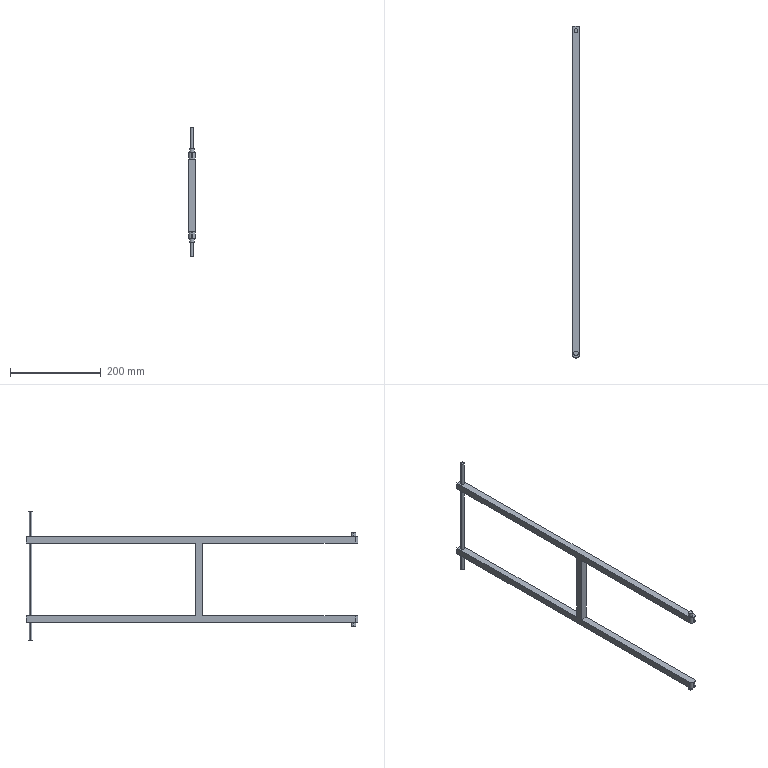Part | SolidWorks | features ICE 5, Extrusion 1, Fillet 1 | 1 solid | 32 faces | box 15 x 730 x 285 mm | volume 378111 mm3 | plane 18 | cylinder 14 | commonest cylinder face diameters 8 x6 10 x4 12 x4
STEP:
#1=CARTESIAN_POINT('',(4.,720.,-47.5));
#2=VERTEX_POINT('',#1);
#3=CARTESIAN_POINT('',(-4.,720.,-47.5));
#4=VERTEX_POINT('',#3);
#5=CARTESIAN_POINT('',(0.,720.,-47.5));
#6=DIRECTION('',(0.,0.,1.));
#7=DIRECTION('',(1.,0.,0.));
#8=AXIS2_PLACEMENT_3D('',#5,#6,#7);
#9=CIRCLE('',#8,4.);
#10=EDGE_CURVE('',#2,#4,#9,.T.);
#11=ORIENTED_EDGE('',*,*,#10,.T.);
#12=CARTESIAN_POINT('',(-4.,720.,-7.5));
#13=VERTEX_POINT('',#12);
#14=CARTESIAN_POINT('',(-4.,720.,-47.5));
#15=DIRECTION('',(0.,0.,1.));
#16=VECTOR('',#15,1000.);
#17=LINE('',#14,#16);
#18=EDGE_CURVE('',#4,#13,#17,.T.);
#19=ORIENTED_EDGE('',*,*,#18,.T.);
#20=CARTESIAN_POINT('',(4.,720.,-7.5));
#21=VERTEX_POINT('',#20);
#22=CARTESIAN_POINT('',(0.,720.,-7.5));
#23=DIRECTION('',(0.,0.,1.));
#24=DIRECTION('',(1.,0.,0.));
#25=AXIS2_PLACEMENT_3D('',#22,#23,#24);
#26=CIRCLE('',#25,4.);
#27=EDGE_CURVE('',#21,#13,#26,.T.);
#28=ORIENTED_EDGE('',*,*,#27,.F.);
#29=CARTESIAN_POINT('',(4.,720.,-47.5));
#30=DIRECTION('',(0.,0.,1.));
#31=VECTOR('',#30,1000.);
#32=LINE('',#29,#31);
#33=EDGE_CURVE('',#2,#21,#32,.T.);
#34=ORIENTED_EDGE('',*,*,#33,.F.);
#35=EDGE_LOOP('',(#11,#19,#28,#34));
#36=FACE_OUTER_BOUND('',#35,.T.);
#37=CARTESIAN_POINT('',(0.,720.,-47.5));
#38=DIRECTION('',(0.,0.,1.));
#39=DIRECTION('',(1.,0.,0.));
#40=AXIS2_PLACEMENT_3D('',#37,#38,#39);
#41=CYLINDRICAL_SURFACE('',#40,4.);
#42=ADVANCED_FACE('',(#36),#41,.T.);
#43=CARTESIAN_POINT('',(-4.,720.,7.5));
#44=VERTEX_POINT('',#43);
#45=CARTESIAN_POINT('',(4.,720.,7.5));
#46=VERTEX_POINT('',#45);
#47=CARTESIAN_POINT('',(0.,720.,7.5));
#48=DIRECTION('',(0.,0.,-1.));
#49=DIRECTION('',(-1.,0.,0.));
#50=AXIS2_PLACEMENT_3D('',#47,#48,#49);
#51=CIRCLE('',#50,4.);
#52=EDGE_CURVE('',#44,#46,#51,.T.);
#53=ORIENTED_EDGE('',*,*,#52,.F.);
#54=CARTESIAN_POINT('',(-4.,720.,167.5));
#55=VERTEX_POINT('',#54);
#56=CARTESIAN_POINT('',(-4.,720.,-47.5));
#57=DIRECTION('',(0.,0.,1.));
#58=VECTOR('',#57,1000.);
#59=LINE('',#56,#58);
#60=EDGE_CURVE('',#44,#55,#59,.T.);
#61=ORIENTED_EDGE('',*,*,#60,.T.);
#62=CARTESIAN_POINT('',(4.,720.,167.5));
#63=VERTEX_POINT('',#62);
#64=CARTESIAN_POINT('',(0.,720.,167.5));
#65=DIRECTION('',(0.,0.,1.));
#66=DIRECTION('',(1.,0.,0.));
#67=AXIS2_PLACEMENT_3D('',#64,#65,#66);
#68=CIRCLE('',#67,4.);
#69=EDGE_CURVE('',#63,#55,#68,.T.);
#70=ORIENTED_EDGE('',*,*,#69,.F.);
#71=CARTESIAN_POINT('',(4.,720.,-47.5));
#72=DIRECTION('',(0.,0.,1.));
#73=VECTOR('',#72,1000.);
#74=LINE('',#71,#73);
#75=EDGE_CURVE('',#46,#63,#74,.T.);
#76=ORIENTED_EDGE('',*,*,#75,.F.);
#77=EDGE_LOOP('',(#53,#61,#70,#76));
#78=FACE_OUTER_BOUND('',#77,.T.);
#79=CARTESIAN_POINT('',(0.,720.,-47.5));
#80=DIRECTION('',(0.,0.,1.));
#81=DIRECTION('',(1.,0.,0.));
#82=AXIS2_PLACEMENT_3D('',#79,#80,#81);
#83=CYLINDRICAL_SURFACE('',#82,4.);
#84=ADVANCED_FACE('',(#78),#83,.T.);
#85=CARTESIAN_POINT('',(4.,720.,182.5));
#86=VERTEX_POINT('',#85);
#87=CARTESIAN_POINT('',(-4.,720.,182.5));
#88=VERTEX_POINT('',#87);
#89=CARTESIAN_POINT('',(0.,720.,182.5));
#90=DIRECTION('',(0.,0.,1.));
#91=DIRECTION('',(1.,0.,0.));
#92=AXIS2_PLACEMENT_3D('',#89,#90,#91);
#93=CIRCLE('',#92,4.);
#94=EDGE_CURVE('',#86,#88,#93,.T.);
#95=ORIENTED_EDGE('',*,*,#94,.T.);
#96=CARTESIAN_POINT('',(-4.,720.,237.5));
#97=VERTEX_POINT('',#96);
#98=CARTESIAN_POINT('',(-4.,720.,-47.5));
#99=DIRECTION('',(0.,0.,1.));
#100=VECTOR('',#99,1000.);
#101=LINE('',#98,#100);
#102=EDGE_CURVE('',#88,#97,#101,.T.);
#103=ORIENTED_EDGE('',*,*,#102,.T.);
#104=CARTESIAN_POINT('',(4.,720.,237.5));
#105=VERTEX_POINT('',#104);
#106=CARTESIAN_POINT('',(0.,720.,237.5));
#107=DIRECTION('',(0.,0.,1.));
#108=DIRECTION('',(1.,0.,0.));
#109=AXIS2_PLACEMENT_3D('',#106,#107,#108);
#110=CIRCLE('',#109,4.);
#111=EDGE_CURVE('',#105,#97,#110,.T.);
#112=ORIENTED_EDGE('',*,*,#111,.F.);
#113=CARTESIAN_POINT('',(4.,720.,-47.5));
#114=DIRECTION('',(0.,0.,1.));
#115=VECTOR('',#114,1000.);
#116=LINE('',#113,#115);
#117=EDGE_CURVE('',#86,#105,#116,.T.);
#118=ORIENTED_EDGE('',*,*,#117,.F.);
#119=EDGE_LOOP('',(#95,#103,#112,#118));
#120=FACE_OUTER_BOUND('',#119,.T.);
#121=CARTESIAN_POINT('',(0.,720.,-47.5));
#122=DIRECTION('',(0.,0.,1.));
#123=DIRECTION('',(1.,0.,0.));
#124=AXIS2_PLACEMENT_3D('',#121,#122,#123);
#125=CYLINDRICAL_SURFACE('',#124,4.);
#126=ADVANCED_FACE('',(#120),#125,.T.);
#127=CARTESIAN_POINT('',(5.,10.,190.5));
#128=VERTEX_POINT('',#127);
#129=CARTESIAN_POINT('',(-5.,10.,190.5));
#130=VERTEX_POINT('',#129);
#131=CARTESIAN_POINT('',(0.,10.,190.5));
#132=DIRECTION('',(0.,0.,1.));
#133=DIRECTION('',(1.,0.,0.));
#134=AXIS2_PLACEMENT_3D('',#131,#132,#133);
#135=CIRCLE('',#134,5.);
#136=EDGE_CURVE('',#128,#130,#135,.T.);
#137=ORIENTED_EDGE('',*,*,#136,.F.);
#138=CARTESIAN_POINT('',(5.,10.,182.5));
#139=VERTEX_POINT('',#138);
#140=CARTESIAN_POINT('',(5.,10.,190.5));
#141=DIRECTION('',(0.,0.,-1.));
#142=VECTOR('',#141,1000.);
#143=LINE('',#140,#142);
#144=EDGE_CURVE('',#128,#139,#143,.T.);
#145=ORIENTED_EDGE('',*,*,#144,.T.);
#146=CARTESIAN_POINT('',(-5.,10.,182.5));
#147=VERTEX_POINT('',#146);
#148=CARTESIAN_POINT('',(0.,10.,182.5));
#149=DIRECTION('',(0.,0.,1.));
#150=DIRECTION('',(1.,0.,0.));
#151=AXIS2_PLACEMENT_3D('',#148,#149,#150);
#152=CIRCLE('',#151,5.);
#153=EDGE_CURVE('',#139,#147,#152,.T.);
#154=ORIENTED_EDGE('',*,*,#153,.T.);
#155=CARTESIAN_POINT('',(-5.,10.,190.5));
#156=DIRECTION('',(0.,0.,-1.));
#157=VECTOR('',#156,1000.);
#158=LINE('',#155,#157);
#159=EDGE_CURVE('',#130,#147,#158,.T.);
#160=ORIENTED_EDGE('',*,*,#159,.F.);
#161=EDGE_LOOP('',(#137,#145,#154,#160));
#162=FACE_OUTER_BOUND('',#161,.T.);
#163=CARTESIAN_POINT('',(0.,10.,190.5));
#164=DIRECTION('',(0.,0.,-1.));
#165=DIRECTION('',(-1.,0.,0.));
#166=AXIS2_PLACEMENT_3D('',#163,#164,#165);
#167=CYLINDRICAL_SURFACE('',#166,5.);
#168=ADVANCED_FACE('',(#162),#167,.T.);
#169=CARTESIAN_POINT('',(-5.,10.,-15.5));
#170=VERTEX_POINT('',#169);
#171=CARTESIAN_POINT('',(5.,10.,-15.5));
#172=VERTEX_POINT('',#171);
#173=CARTESIAN_POINT('',(0.,10.,-15.5));
#174=DIRECTION('',(0.,0.,-1.));
#175=DIRECTION('',(-1.,0.,0.));
#176=AXIS2_PLACEMENT_3D('',#173,#174,#175);
#177=CIRCLE('',#176,5.);
#178=EDGE_CURVE('',#170,#172,#177,.T.);
#179=ORIENTED_EDGE('',*,*,#178,.F.);
#180=CARTESIAN_POINT('',(-5.,10.,-7.5));
#181=VERTEX_POINT('',#180);
#182=CARTESIAN_POINT('',(-5.,10.,-15.5));
#183=DIRECTION('',(0.,0.,1.));
#184=VECTOR('',#183,1000.);
#185=LINE('',#182,#184);
#186=EDGE_CURVE('',#170,#181,#185,.T.);
#187=ORIENTED_EDGE('',*,*,#186,.T.);
#188=CARTESIAN_POINT('',(5.,10.,-7.5));
#189=VERTEX_POINT('',#188);
#190=CARTESIAN_POINT('',(0.,10.,-7.5));
#191=DIRECTION('',(0.,0.,-1.));
#192=DIRECTION('',(1.,0.,0.));
#193=AXIS2_PLACEMENT_3D('',#190,#191,#192);
#194=CIRCLE('',#193,5.);
#195=EDGE_CURVE('',#181,#189,#194,.T.);
#196=ORIENTED_EDGE('',*,*,#195,.T.);
#197=CARTESIAN_POINT('',(5.,10.,-15.5));
#198=DIRECTION('',(0.,0.,1.));
#199=VECTOR('',#198,1000.);
#200=LINE('',#197,#199);
#201=EDGE_CURVE('',#172,#189,#200,.T.);
#202=ORIENTED_EDGE('',*,*,#201,.F.);
#203=EDGE_LOOP('',(#179,#187,#196,#202));
#204=FACE_OUTER_BOUND('',#203,.T.);
#205=CARTESIAN_POINT('',(0.,10.,-15.5));
#206=DIRECTION('',(0.,0.,1.));
#207=DIRECTION('',(1.,0.,0.));
#208=AXIS2_PLACEMENT_3D('',#205,#206,#207);
#209=CYLINDRICAL_SURFACE('',#208,5.);
#210=ADVANCED_FACE('',(#204),#209,.T.);
#211=CARTESIAN_POINT('',(-7.5,342.5,7.5));
#212=VERTEX_POINT('',#211);
#213=CARTESIAN_POINT('',(-7.5,6.,7.5));
#214=VERTEX_POINT('',#213);
#215=CARTESIAN_POINT('',(-7.5,730.,7.5));
#216=DIRECTION('',(0.,-1.,0.));
#217=VECTOR('',#216,1000.);
#218=LINE('',#215,#217);
#219=EDGE_CURVE('',#212,#214,#218,.T.);
#220=ORIENTED_EDGE('',*,*,#219,.T.);
#221=CARTESIAN_POINT('',(-1.5,0.,7.5));
#222=VERTEX_POINT('',#221);
#223=CARTESIAN_POINT('',(-1.5,6.,7.5));
#224=DIRECTION('',(0.,0.,1.));
#225=DIRECTION('',(-1.,0.,0.));
#226=AXIS2_PLACEMENT_3D('',#223,#224,#225);
#227=CIRCLE('',#226,6.);
#228=EDGE_CURVE('',#214,#222,#227,.T.);
#229=ORIENTED_EDGE('',*,*,#228,.T.);
#230=CARTESIAN_POINT('',(1.5,0.,7.5));
#231=VERTEX_POINT('',#230);
#232=CARTESIAN_POINT('',(-7.5,0.,7.5));
#233=DIRECTION('',(1.,0.,0.));
#234=VECTOR('',#233,1000.);
#235=LINE('',#232,#234);
#236=EDGE_CURVE('',#222,#231,#235,.T.);
#237=ORIENTED_EDGE('',*,*,#236,.T.);
#238=CARTESIAN_POINT('',(7.5,6.,7.5));
#239=VERTEX_POINT('',#238);
#240=CARTESIAN_POINT('',(1.5,6.,7.5));
#241=DIRECTION('',(0.,0.,1.));
#242=DIRECTION('',(-1.,0.,0.));
#243=AXIS2_PLACEMENT_3D('',#240,#241,#242);
#244=CIRCLE('',#243,6.);
#245=EDGE_CURVE('',#231,#239,#244,.T.);
#246=ORIENTED_EDGE('',*,*,#245,.T.);
#247=CARTESIAN_POINT('',(7.5,342.5,7.5));
#248=VERTEX_POINT('',#247);
#249=CARTESIAN_POINT('',(7.5,730.,7.5));
#250=DIRECTION('',(0.,-1.,0.));
#251=VECTOR('',#250,1000.);
#252=LINE('',#249,#251);
#253=EDGE_CURVE('',#248,#239,#252,.T.);
#254=ORIENTED_EDGE('',*,*,#253,.F.);
#255=CARTESIAN_POINT('',(-7.5,342.5,7.5));
#256=DIRECTION('',(1.,0.,0.));
#257=VECTOR('',#256,1000.);
#258=LINE('',#255,#257);
#259=EDGE_CURVE('',#212,#248,#258,.T.);
#260=ORIENTED_EDGE('',*,*,#259,.F.);
#261=EDGE_LOOP('',(#220,#229,#237,#246,#254,#260));
#262=FACE_OUTER_BOUND('',#261,.T.);
#263=CARTESIAN_POINT('',(-7.5,730.,7.5));
#264=DIRECTION('',(0.,0.,-1.));
#265=DIRECTION('',(-1.,0.,0.));
#266=AXIS2_PLACEMENT_3D('',#263,#264,#265);
#267=PLANE('',#266);
#268=ADVANCED_FACE('',(#262),#267,.F.);
#269=CARTESIAN_POINT('',(0.,720.,7.5));
#270=DIRECTION('',(0.,0.,-1.));
#271=DIRECTION('',(-1.,0.,0.));
#272=AXIS2_PLACEMENT_3D('',#269,#270,#271);
#273=CIRCLE('',#272,4.);
#274=EDGE_CURVE('',#46,#44,#273,.T.);
#275=ORIENTED_EDGE('',*,*,#274,.T.);
#276=ORIENTED_EDGE('',*,*,#52,.T.);
#277=EDGE_LOOP('',(#275,#276));
#278=FACE_BOUND('',#277,.T.);
#279=CARTESIAN_POINT('',(7.5,357.5,7.5));
#280=VERTEX_POINT('',#279);
#281=CARTESIAN_POINT('',(-7.5,357.5,7.5));
#282=VERTEX_POINT('',#281);
#283=CARTESIAN_POINT('',(-7.5,357.5,7.5));
#284=DIRECTION('',(-1.,0.,0.));
#285=VECTOR('',#284,1000.);
#286=LINE('',#283,#285);
#287=EDGE_CURVE('',#280,#282,#286,.T.);
#288=ORIENTED_EDGE('',*,*,#287,.F.);
#289=CARTESIAN_POINT('',(7.5,730.,7.5));
#290=VERTEX_POINT('',#289);
#291=CARTESIAN_POINT('',(7.5,730.,7.5));
#292=DIRECTION('',(0.,-1.,0.));
#293=VECTOR('',#292,1000.);
#294=LINE('',#291,#293);
#295=EDGE_CURVE('',#290,#280,#294,.T.);
#296=ORIENTED_EDGE('',*,*,#295,.F.);
#297=CARTESIAN_POINT('',(-7.5,730.,7.5));
#298=VERTEX_POINT('',#297);
#299=CARTESIAN_POINT('',(-7.5,730.,7.5));
#300=DIRECTION('',(1.,0.,0.));
#301=VECTOR('',#300,1000.);
#302=LINE('',#299,#301);
#303=EDGE_CURVE('',#298,#290,#302,.T.);
#304=ORIENTED_EDGE('',*,*,#303,.F.);
#305=CARTESIAN_POINT('',(-7.5,730.,7.5));
#306=DIRECTION('',(0.,-1.,0.));
#307=VECTOR('',#306,1000.);
#308=LINE('',#305,#307);
#309=EDGE_CURVE('',#298,#282,#308,.T.);
#310=ORIENTED_EDGE('',*,*,#309,.T.);
#311=EDGE_LOOP('',(#288,#296,#304,#310));
#312=FACE_OUTER_BOUND('',#311,.T.);
#313=CARTESIAN_POINT('',(-7.5,730.,7.5));
#314=DIRECTION('',(0.,0.,-1.));
#315=DIRECTION('',(-1.,0.,0.));
#316=AXIS2_PLACEMENT_3D('',#313,#314,#315);
#317=PLANE('',#316);
#318=ADVANCED_FACE('',(#278,#312),#317,.F.);
#319=CARTESIAN_POINT('',(7.5,6.,182.5));
#320=VERTEX_POINT('',#319);
#321=CARTESIAN_POINT('',(7.5,730.,182.5));
#322=VERTEX_POINT('',#321);
#323=CARTESIAN_POINT('',(7.5,730.,182.5));
#324=DIRECTION('',(0.,1.,0.));
#325=VECTOR('',#324,1000.);
#326=LINE('',#323,#325);
#327=EDGE_CURVE('',#320,#322,#326,.T.);
#328=ORIENTED_EDGE('',*,*,#327,.F.);
#329=CARTESIAN_POINT('',(7.5,6.,167.5));
#330=VERTEX_POINT('',#329);
#331=CARTESIAN_POINT('',(7.5,6.,-7.5));
#332=DIRECTION('',(0.,0.,-1.));
#333=VECTOR('',#332,1000.);
#334=LINE('',#331,#333);
#335=EDGE_CURVE('',#320,#330,#334,.T.);
#336=ORIENTED_EDGE('',*,*,#335,.T.);
#337=CARTESIAN_POINT('',(7.5,342.5,167.5));
#338=VERTEX_POINT('',#337);
#339=CARTESIAN_POINT('',(7.5,730.,167.5));
#340=DIRECTION('',(0.,1.,0.));
#341=VECTOR('',#340,1000.);
#342=LINE('',#339,#341);
#343=EDGE_CURVE('',#330,#338,#342,.T.);
#344=ORIENTED_EDGE('',*,*,#343,.T.);
#345=CARTESIAN_POINT('',(7.5,342.5,167.5));
#346=DIRECTION('',(0.,0.,-1.));
#347=VECTOR('',#346,1000.);
#348=LINE('',#345,#347);
#349=EDGE_CURVE('',#338,#248,#348,.T.);
#350=ORIENTED_EDGE('',*,*,#349,.T.);
#351=ORIENTED_EDGE('',*,*,#253,.T.);
#352=CARTESIAN_POINT('',(7.5,6.,-7.5));
#353=VERTEX_POINT('',#352);
#354=CARTESIAN_POINT('',(7.5,6.,-7.5));
#355=DIRECTION('',(0.,0.,-1.));
#356=VECTOR('',#355,1000.);
#357=LINE('',#354,#356);
#358=EDGE_CURVE('',#239,#353,#357,.T.);
#359=ORIENTED_EDGE('',*,*,#358,.T.);
#360=CARTESIAN_POINT('',(7.5,730.,-7.5));
#361=VERTEX_POINT('',#360);
#362=CARTESIAN_POINT('',(7.5,730.,-7.5));
#363=DIRECTION('',(0.,-1.,0.));
#364=VECTOR('',#363,1000.);
#365=LINE('',#362,#364);
#366=EDGE_CURVE('',#361,#353,#365,.T.);
#367=ORIENTED_EDGE('',*,*,#366,.F.);
#368=CARTESIAN_POINT('',(7.5,730.,-7.5));
#369=DIRECTION('',(0.,0.,-1.));
#370=VECTOR('',#369,1000.);
#371=LINE('',#368,#370);
#372=EDGE_CURVE('',#290,#361,#371,.T.);
#373=ORIENTED_EDGE('',*,*,#372,.F.);
#374=ORIENTED_EDGE('',*,*,#295,.T.);
#375=CARTESIAN_POINT('',(7.5,357.5,167.5));
#376=VERTEX_POINT('',#375);
#377=CARTESIAN_POINT('',(7.5,357.5,167.5));
#378=DIRECTION('',(0.,0.,-1.));
#379=VECTOR('',#378,1000.);
#380=LINE('',#377,#379);
#381=EDGE_CURVE('',#376,#280,#380,.T.);
#382=ORIENTED_EDGE('',*,*,#381,.F.);
#383=CARTESIAN_POINT('',(7.5,730.,167.5));
#384=VERTEX_POINT('',#383);
#385=CARTESIAN_POINT('',(7.5,730.,167.5));
#386=DIRECTION('',(0.,1.,0.));
#387=VECTOR('',#386,1000.);
#388=LINE('',#385,#387);
#389=EDGE_CURVE('',#376,#384,#388,.T.);
#390=ORIENTED_EDGE('',*,*,#389,.T.);
#391=CARTESIAN_POINT('',(7.5,730.,182.5));
#392=DIRECTION('',(0.,0.,-1.));
#393=VECTOR('',#392,1000.);
#394=LINE('',#391,#393);
#395=EDGE_CURVE('',#322,#384,#394,.T.);
#396=ORIENTED_EDGE('',*,*,#395,.F.);
#397=EDGE_LOOP('',(#328,#336,#344,#350,#351,#359,#367,#373,#374,#382,#390,#396));
#398=FACE_OUTER_BOUND('',#397,.T.);
#399=CARTESIAN_POINT('',(7.5,730.,-7.5));
#400=DIRECTION('',(-1.,0.,0.));
#401=DIRECTION('',(0.,0.,1.));
#402=AXIS2_PLACEMENT_3D('',#399,#400,#401);
#403=PLANE('',#402);
#404=ADVANCED_FACE('',(#398),#403,.F.);
#405=ORIENTED_EDGE('',*,*,#27,.T.);
#406=CARTESIAN_POINT('',(0.,720.,-7.5));
#407=DIRECTION('',(0.,0.,1.));
#408=DIRECTION('',(1.,0.,0.));
#409=AXIS2_PLACEMENT_3D('',#406,#407,#408);
#410=CIRCLE('',#409,4.);
#411=EDGE_CURVE('',#13,#21,#410,.T.);
#412=ORIENTED_EDGE('',*,*,#411,.T.);
#413=EDGE_LOOP('',(#405,#412));
#414=FACE_BOUND('',#413,.T.);
#415=CARTESIAN_POINT('',(0.,10.,-7.5));
#416=DIRECTION('',(0.,0.,-1.));
#417=DIRECTION('',(1.,0.,0.));
#418=AXIS2_PLACEMENT_3D('',#415,#416,#417);
#419=CIRCLE('',#418,5.);
#420=EDGE_CURVE('',#189,#181,#419,.T.);
#421=ORIENTED_EDGE('',*,*,#420,.F.);
#422=ORIENTED_EDGE('',*,*,#195,.F.);
#423=EDGE_LOOP('',(#421,#422));
#424=FACE_BOUND('',#423,.T.);
#425=CARTESIAN_POINT('',(1.5,0.,-7.5));
#426=VERTEX_POINT('',#425);
#427=CARTESIAN_POINT('',(-1.5,0.,-7.5));
#428=VERTEX_POINT('',#427);
#429=CARTESIAN_POINT('',(-7.5,0.,-7.5));
#430=DIRECTION('',(-1.,0.,0.));
#431=VECTOR('',#430,1000.);
#432=LINE('',#429,#431);
#433=EDGE_CURVE('',#426,#428,#432,.T.);
#434=ORIENTED_EDGE('',*,*,#433,.T.);
#435=CARTESIAN_POINT('',(-7.5,6.,-7.5));
#436=VERTEX_POINT('',#435);
#437=CARTESIAN_POINT('',(-1.5,6.,-7.5));
#438=DIRECTION('',(0.,0.,-1.));
#439=DIRECTION('',(1.,0.,0.));
#440=AXIS2_PLACEMENT_3D('',#437,#438,#439);
#441=CIRCLE('',#440,6.);
#442=EDGE_CURVE('',#428,#436,#441,.T.);
#443=ORIENTED_EDGE('',*,*,#442,.T.);
#444=CARTESIAN_POINT('',(-7.5,730.,-7.5));
#445=VERTEX_POINT('',#444);
#446=CARTESIAN_POINT('',(-7.5,730.,-7.5));
#447=DIRECTION('',(0.,-1.,0.));
#448=VECTOR('',#447,1000.);
#449=LINE('',#446,#448);
#450=EDGE_CURVE('',#445,#436,#449,.T.);
#451=ORIENTED_EDGE('',*,*,#450,.F.);
#452=CARTESIAN_POINT('',(-7.5,730.,-7.5));
#453=DIRECTION('',(-1.,0.,0.));
#454=VECTOR('',#453,1000.);
#455=LINE('',#452,#454);
#456=EDGE_CURVE('',#361,#445,#455,.T.);
#457=ORIENTED_EDGE('',*,*,#456,.F.);
#458=ORIENTED_EDGE('',*,*,#366,.T.);
#459=CARTESIAN_POINT('',(1.5,6.,-7.5));
#460=DIRECTION('',(0.,0.,-1.));
#461=DIRECTION('',(1.,0.,0.));
#462=AXIS2_PLACEMENT_3D('',#459,#460,#461);
#463=CIRCLE('',#462,6.);
#464=EDGE_CURVE('',#353,#426,#463,.T.);
#465=ORIENTED_EDGE('',*,*,#464,.T.);
#466=EDGE_LOOP('',(#434,#443,#451,#457,#458,#465));
#467=FACE_OUTER_BOUND('',#466,.T.);
#468=CARTESIAN_POINT('',(-7.5,730.,-7.5));
#469=DIRECTION('',(0.,0.,1.));
#470=DIRECTION('',(1.,0.,0.));
#471=AXIS2_PLACEMENT_3D('',#468,#469,#470);
#472=PLANE('',#471);
#473=ADVANCED_FACE('',(#414,#424,#467),#472,.F.);
#474=CARTESIAN_POINT('',(-7.5,342.5,167.5));
#475=VERTEX_POINT('',#474);
#476=CARTESIAN_POINT('',(-7.5,6.,167.5));
#477=VERTEX_POINT('',#476);
#478=CARTESIAN_POINT('',(-7.5,730.,167.5));
#479=DIRECTION('',(0.,-1.,0.));
#480=VECTOR('',#479,1000.);
#481=LINE('',#478,#480);
#482=EDGE_CURVE('',#475,#477,#481,.T.);
#483=ORIENTED_EDGE('',*,*,#482,.T.);
#484=CARTESIAN_POINT('',(-7.5,6.,182.5));
#485=VERTEX_POINT('',#484);
#486=CARTESIAN_POINT('',(-7.5,6.,-7.5));
#487=DIRECTION('',(0.,0.,1.));
#488=VECTOR('',#487,1000.);
#489=LINE('',#486,#488);
#490=EDGE_CURVE('',#477,#485,#489,.T.);
#491=ORIENTED_EDGE('',*,*,#490,.T.);
#492=CARTESIAN_POINT('',(-7.5,730.,182.5));
#493=VERTEX_POINT('',#492);
#494=CARTESIAN_POINT('',(-7.5,730.,182.5));
#495=DIRECTION('',(0.,-1.,0.));
#496=VECTOR('',#495,1000.);
#497=LINE('',#494,#496);
#498=EDGE_CURVE('',#493,#485,#497,.T.);
#499=ORIENTED_EDGE('',*,*,#498,.F.);
#500=CARTESIAN_POINT('',(-7.5,730.,167.5));
#501=VERTEX_POINT('',#500);
#502=CARTESIAN_POINT('',(-7.5,730.,182.5));
#503=DIRECTION('',(0.,0.,-1.));
#504=VECTOR('',#503,1000.);
#505=LINE('',#502,#504);
#506=EDGE_CURVE('',#493,#501,#505,.T.);
#507=ORIENTED_EDGE('',*,*,#506,.T.);
#508=CARTESIAN_POINT('',(-7.5,357.5,167.5));
#509=VERTEX_POINT('',#508);
#510=CARTESIAN_POINT('',(-7.5,730.,167.5));
#511=DIRECTION('',(0.,-1.,0.));
#512=VECTOR('',#511,1000.);
#513=LINE('',#510,#512);
#514=EDGE_CURVE('',#501,#509,#513,.T.);
#515=ORIENTED_EDGE('',*,*,#514,.T.);
#516=CARTESIAN_POINT('',(-7.5,357.5,167.5));
#517=DIRECTION('',(0.,0.,-1.));
#518=VECTOR('',#517,1000.);
#519=LINE('',#516,#518);
#520=EDGE_CURVE('',#509,#282,#519,.T.);
#521=ORIENTED_EDGE('',*,*,#520,.T.);
#522=ORIENTED_EDGE('',*,*,#309,.F.);
#523=CARTESIAN_POINT('',(-7.5,730.,-7.5));
#524=DIRECTION('',(0.,0.,1.));
#525=VECTOR('',#524,1000.);
#526=LINE('',#523,#525);
#527=EDGE_CURVE('',#445,#298,#526,.T.);
#528=ORIENTED_EDGE('',*,*,#527,.F.);
#529=ORIENTED_EDGE('',*,*,#450,.T.);
#530=CARTESIAN_POINT('',(-7.5,6.,-7.5));
#531=DIRECTION('',(0.,0.,1.));
#532=VECTOR('',#531,1000.);
#533=LINE('',#530,#532);
#534=EDGE_CURVE('',#436,#214,#533,.T.);
#535=ORIENTED_EDGE('',*,*,#534,.T.);
#536=ORIENTED_EDGE('',*,*,#219,.F.);
#537=CARTESIAN_POINT('',(-7.5,342.5,167.5));
#538=DIRECTION('',(0.,0.,-1.));
#539=VECTOR('',#538,1000.);
#540=LINE('',#537,#539);
#541=EDGE_CURVE('',#475,#212,#540,.T.);
#542=ORIENTED_EDGE('',*,*,#541,.F.);
#543=EDGE_LOOP('',(#483,#491,#499,#507,#515,#521,#522,#528,#529,#535,#536,#542));
#544=FACE_OUTER_BOUND('',#543,.T.);
#545=CARTESIAN_POINT('',(-7.5,730.,-7.5));
#546=DIRECTION('',(1.,0.,0.));
#547=DIRECTION('',(0.,0.,-1.));
#548=AXIS2_PLACEMENT_3D('',#545,#546,#547);
#549=PLANE('',#548);
#550=ADVANCED_FACE('',(#544),#549,.F.);
#551=ORIENTED_EDGE('',*,*,#372,.T.);
#552=ORIENTED_EDGE('',*,*,#456,.T.);
#553=ORIENTED_EDGE('',*,*,#527,.T.);
#554=ORIENTED_EDGE('',*,*,#303,.T.);
#555=EDGE_LOOP('',(#551,#552,#553,#554));
#556=FACE_OUTER_BOUND('',#555,.T.);
#557=CARTESIAN_POINT('',(0.,730.,0.));
#558=DIRECTION('',(0.,1.,0.));
#559=DIRECTION('',(0.,0.,1.));
#560=AXIS2_PLACEMENT_3D('',#557,#558,#559);
#561=PLANE('',#560);
#562=ADVANCED_FACE('',(#556),#561,.T.);
#563=ORIENTED_EDGE('',*,*,#236,.F.);
#564=CARTESIAN_POINT('',(-1.5,0.,0.));
#565=DIRECTION('',(0.,0.,-1.));
#566=VECTOR('',#565,1000.);
#567=LINE('',#564,#566);
#568=EDGE_CURVE('',#222,#428,#567,.T.);
#569=ORIENTED_EDGE('',*,*,#568,.T.);
#570=ORIENTED_EDGE('',*,*,#433,.F.);
#571=CARTESIAN_POINT('',(1.5,0.,0.));
#572=DIRECTION('',(0.,0.,1.));
#573=VECTOR('',#572,1000.);
#574=LINE('',#571,#573);
#575=EDGE_CURVE('',#426,#231,#574,.T.);
#576=ORIENTED_EDGE('',*,*,#575,.T.);
#577=EDGE_LOOP('',(#563,#569,#570,#576));
#578=FACE_OUTER_BOUND('',#577,.T.);
#579=CARTESIAN_POINT('',(0.,0.,0.));
#580=DIRECTION('',(0.,1.,0.));
#581=DIRECTION('',(0.,0.,1.));
#582=AXIS2_PLACEMENT_3D('',#579,#580,#581);
#583=PLANE('',#582);
#584=ADVANCED_FACE('',(#578),#583,.F.);
#585=ORIENTED_EDGE('',*,*,#186,.F.);
#586=CARTESIAN_POINT('',(0.,10.,-15.5));
#587=DIRECTION('',(0.,0.,-1.));
#588=DIRECTION('',(-1.,0.,0.));
#589=AXIS2_PLACEMENT_3D('',#586,#587,#588);
#590=CIRCLE('',#589,5.);
#591=EDGE_CURVE('',#172,#170,#590,.T.);
#592=ORIENTED_EDGE('',*,*,#591,.F.);
#593=ORIENTED_EDGE('',*,*,#201,.T.);
#594=ORIENTED_EDGE('',*,*,#420,.T.);
#595=EDGE_LOOP('',(#585,#592,#593,#594));
#596=FACE_OUTER_BOUND('',#595,.T.);
#597=CARTESIAN_POINT('',(0.,10.,-15.5));
#598=DIRECTION('',(0.,0.,1.));
#599=DIRECTION('',(1.,0.,0.));
#600=AXIS2_PLACEMENT_3D('',#597,#598,#599);
#601=CYLINDRICAL_SURFACE('',#600,5.);
#602=ADVANCED_FACE('',(#596),#601,.T.);
#603=ORIENTED_EDGE('',*,*,#591,.T.);
#604=ORIENTED_EDGE('',*,*,#178,.T.);
#605=EDGE_LOOP('',(#603,#604));
#606=FACE_OUTER_BOUND('',#605,.T.);
#607=CARTESIAN_POINT('',(0.,10.,-15.5));
#608=DIRECTION('',(0.,0.,-1.));
#609=DIRECTION('',(-1.,0.,0.));
#610=AXIS2_PLACEMENT_3D('',#607,#608,#609);
#611=PLANE('',#610);
#612=ADVANCED_FACE('',(#606),#611,.T.);
#613=ORIENTED_EDGE('',*,*,#287,.T.);
#614=ORIENTED_EDGE('',*,*,#520,.F.);
#615=CARTESIAN_POINT('',(-7.5,357.5,167.5));
#616=DIRECTION('',(-1.,0.,0.));
#617=VECTOR('',#616,1000.);
#618=LINE('',#615,#617);
#619=EDGE_CURVE('',#376,#509,#618,.T.);
#620=ORIENTED_EDGE('',*,*,#619,.F.);
#621=ORIENTED_EDGE('',*,*,#381,.T.);
#622=EDGE_LOOP('',(#613,#614,#620,#621));
#623=FACE_OUTER_BOUND('',#622,.T.);
#624=CARTESIAN_POINT('',(-7.5,357.5,167.5));
#625=DIRECTION('',(0.,-1.,0.));
#626=DIRECTION('',(0.,0.,-1.));
#627=AXIS2_PLACEMENT_3D('',#624,#625,#626);
#628=PLANE('',#627);
#629=ADVANCED_FACE('',(#623),#628,.F.);
#630=ORIENTED_EDGE('',*,*,#259,.T.);
#631=ORIENTED_EDGE('',*,*,#349,.F.);
#632=CARTESIAN_POINT('',(-7.5,342.5,167.5));
#633=DIRECTION('',(1.,0.,0.));
#634=VECTOR('',#633,1000.);
#635=LINE('',#632,#634);
#636=EDGE_CURVE('',#475,#338,#635,.T.);
#637=ORIENTED_EDGE('',*,*,#636,.F.);
#638=ORIENTED_EDGE('',*,*,#541,.T.);
#639=EDGE_LOOP('',(#630,#631,#637,#638));
#640=FACE_OUTER_BOUND('',#639,.T.);
#641=CARTESIAN_POINT('',(-7.5,342.5,167.5));
#642=DIRECTION('',(0.,1.,0.));
#643=DIRECTION('',(0.,0.,1.));
#644=AXIS2_PLACEMENT_3D('',#641,#642,#643);
#645=PLANE('',#644);
#646=ADVANCED_FACE('',(#640),#645,.F.);
#647=ORIENTED_EDGE('',*,*,#69,.T.);
#648=CARTESIAN_POINT('',(0.,720.,167.5));
#649=DIRECTION('',(0.,0.,1.));
#650=DIRECTION('',(1.,0.,0.));
#651=AXIS2_PLACEMENT_3D('',#648,#649,#650);
#652=CIRCLE('',#651,4.);
#653=EDGE_CURVE('',#55,#63,#652,.T.);
#654=ORIENTED_EDGE('',*,*,#653,.T.);
#655=EDGE_LOOP('',(#647,#654));
#656=FACE_BOUND('',#655,.T.);
#657=ORIENTED_EDGE('',*,*,#389,.F.);
#658=ORIENTED_EDGE('',*,*,#619,.T.);
#659=ORIENTED_EDGE('',*,*,#514,.F.);
#660=CARTESIAN_POINT('',(-7.5,730.,167.5));
#661=DIRECTION('',(-1.,0.,0.));
#662=VECTOR('',#661,1000.);
#663=LINE('',#660,#662);
#664=EDGE_CURVE('',#384,#501,#663,.T.);
#665=ORIENTED_EDGE('',*,*,#664,.F.);
#666=EDGE_LOOP('',(#657,#658,#659,#665));
#667=FACE_OUTER_BOUND('',#666,.T.);
#668=CARTESIAN_POINT('',(0.,0.,167.5));
#669=DIRECTION('',(0.,0.,1.));
#670=DIRECTION('',(1.,0.,0.));
#671=AXIS2_PLACEMENT_3D('',#668,#669,#670);
#672=PLANE('',#671);
#673=ADVANCED_FACE('',(#656,#667),#672,.F.);
#674=CARTESIAN_POINT('',(-1.5,0.,167.5));
#675=VERTEX_POINT('',#674);
#676=CARTESIAN_POINT('',(1.5,0.,167.5));
#677=VERTEX_POINT('',#676);
#678=CARTESIAN_POINT('',(-7.5,0.,167.5));
#679=DIRECTION('',(1.,0.,0.));
#680=VECTOR('',#679,1000.);
#681=LINE('',#678,#680);
#682=EDGE_CURVE('',#675,#677,#681,.T.);
#683=ORIENTED_EDGE('',*,*,#682,.F.);
#684=CARTESIAN_POINT('',(-1.5,6.,167.5));
#685=DIRECTION('',(0.,0.,-1.));
#686=DIRECTION('',(1.,0.,0.));
#687=AXIS2_PLACEMENT_3D('',#684,#685,#686);
#688=CIRCLE('',#687,6.);
#689=EDGE_CURVE('',#675,#477,#688,.T.);
#690=ORIENTED_EDGE('',*,*,#689,.T.);
#691=ORIENTED_EDGE('',*,*,#482,.F.);
#692=ORIENTED_EDGE('',*,*,#636,.T.);
#693=ORIENTED_EDGE('',*,*,#343,.F.);
#694=CARTESIAN_POINT('',(1.5,6.,167.5));
#695=DIRECTION('',(0.,0.,-1.));
#696=DIRECTION('',(1.,0.,0.));
#697=AXIS2_PLACEMENT_3D('',#694,#695,#696);
#698=CIRCLE('',#697,6.);
#699=EDGE_CURVE('',#330,#677,#698,.T.);
#700=ORIENTED_EDGE('',*,*,#699,.T.);
#701=EDGE_LOOP('',(#683,#690,#691,#692,#693,#700));
#702=FACE_OUTER_BOUND('',#701,.T.);
#703=CARTESIAN_POINT('',(0.,0.,167.5));
#704=DIRECTION('',(0.,0.,1.));
#705=DIRECTION('',(1.,0.,0.));
#706=AXIS2_PLACEMENT_3D('',#703,#704,#705);
#707=PLANE('',#706);
#708=ADVANCED_FACE('',(#702),#707,.F.);
#709=ORIENTED_EDGE('',*,*,#664,.T.);
#710=ORIENTED_EDGE('',*,*,#506,.F.);
#711=CARTESIAN_POINT('',(-7.5,730.,182.5));
#712=DIRECTION('',(-1.,0.,0.));
#713=VECTOR('',#712,1000.);
#714=LINE('',#711,#713);
#715=EDGE_CURVE('',#322,#493,#714,.T.);
#716=ORIENTED_EDGE('',*,*,#715,.F.);
#717=ORIENTED_EDGE('',*,*,#395,.T.);
#718=EDGE_LOOP('',(#709,#710,#716,#717));
#719=FACE_OUTER_BOUND('',#718,.T.);
#720=CARTESIAN_POINT('',(-7.5,730.,182.5));
#721=DIRECTION('',(0.,-1.,0.));
#722=DIRECTION('',(0.,0.,-1.));
#723=AXIS2_PLACEMENT_3D('',#720,#721,#722);
#724=PLANE('',#723);
#725=ADVANCED_FACE('',(#719),#724,.F.);
#726=CARTESIAN_POINT('',(-1.5,0.,182.5));
#727=VERTEX_POINT('',#726);
#728=CARTESIAN_POINT('',(1.5,0.,182.5));
#729=VERTEX_POINT('',#728);
#730=CARTESIAN_POINT('',(-7.5,0.,182.5));
#731=DIRECTION('',(1.,0.,0.));
#732=VECTOR('',#731,1000.);
#733=LINE('',#730,#732);
#734=EDGE_CURVE('',#727,#729,#733,.T.);
#735=ORIENTED_EDGE('',*,*,#734,.F.);
#736=CARTESIAN_POINT('',(-1.5,0.,182.5));
#737=DIRECTION('',(0.,0.,-1.));
#738=VECTOR('',#737,1000.);
#739=LINE('',#736,#738);
#740=EDGE_CURVE('',#727,#675,#739,.T.);
#741=ORIENTED_EDGE('',*,*,#740,.T.);
#742=ORIENTED_EDGE('',*,*,#682,.T.);
#743=CARTESIAN_POINT('',(1.5,0.,182.5));
#744=DIRECTION('',(0.,0.,1.));
#745=VECTOR('',#744,1000.);
#746=LINE('',#743,#745);
#747=EDGE_CURVE('',#677,#729,#746,.T.);
#748=ORIENTED_EDGE('',*,*,#747,.T.);
#749=EDGE_LOOP('',(#735,#741,#742,#748));
#750=FACE_OUTER_BOUND('',#749,.T.);
#751=CARTESIAN_POINT('',(-7.5,0.,182.5));
#752=DIRECTION('',(0.,1.,0.));
#753=DIRECTION('',(0.,0.,1.));
#754=AXIS2_PLACEMENT_3D('',#751,#752,#753);
#755=PLANE('',#754);
#756=ADVANCED_FACE('',(#750),#755,.F.);
#757=ORIENTED_EDGE('',*,*,#94,.F.);
#758=CARTESIAN_POINT('',(0.,720.,182.5));
#759=DIRECTION('',(0.,0.,1.));
#760=DIRECTION('',(1.,0.,0.));
#761=AXIS2_PLACEMENT_3D('',#758,#759,#760);
#762=CIRCLE('',#761,4.);
#763=EDGE_CURVE('',#88,#86,#762,.T.);
#764=ORIENTED_EDGE('',*,*,#763,.F.);
#765=EDGE_LOOP('',(#757,#764));
#766=FACE_BOUND('',#765,.T.);
#767=CARTESIAN_POINT('',(0.,10.,182.5));
#768=DIRECTION('',(0.,0.,1.));
#769=DIRECTION('',(1.,0.,0.));
#770=AXIS2_PLACEMENT_3D('',#767,#768,#769);
#771=CIRCLE('',#770,5.);
#772=EDGE_CURVE('',#147,#139,#771,.T.);
#773=ORIENTED_EDGE('',*,*,#772,.F.);
#774=ORIENTED_EDGE('',*,*,#153,.F.);
#775=EDGE_LOOP('',(#773,#774));
#776=FACE_BOUND('',#775,.T.);
#777=ORIENTED_EDGE('',*,*,#498,.T.);
#778=CARTESIAN_POINT('',(-1.5,6.,182.5));
#779=DIRECTION('',(0.,0.,1.));
#780=DIRECTION('',(1.,0.,0.));
#781=AXIS2_PLACEMENT_3D('',#778,#779,#780);
#782=CIRCLE('',#781,6.);
#783=EDGE_CURVE('',#485,#727,#782,.T.);
#784=ORIENTED_EDGE('',*,*,#783,.T.);
#785=ORIENTED_EDGE('',*,*,#734,.T.);
#786=CARTESIAN_POINT('',(1.5,6.,182.5));
#787=DIRECTION('',(0.,0.,1.));
#788=DIRECTION('',(1.,0.,0.));
#789=AXIS2_PLACEMENT_3D('',#786,#787,#788);
#790=CIRCLE('',#789,6.);
#791=EDGE_CURVE('',#729,#320,#790,.T.);
#792=ORIENTED_EDGE('',*,*,#791,.T.);
#793=ORIENTED_EDGE('',*,*,#327,.T.);
#794=ORIENTED_EDGE('',*,*,#715,.T.);
#795=EDGE_LOOP('',(#777,#784,#785,#792,#793,#794));
#796=FACE_OUTER_BOUND('',#795,.T.);
#797=CARTESIAN_POINT('',(0.,0.,182.5));
#798=DIRECTION('',(0.,0.,1.));
#799=DIRECTION('',(1.,0.,0.));
#800=AXIS2_PLACEMENT_3D('',#797,#798,#799);
#801=PLANE('',#800);
#802=ADVANCED_FACE('',(#766,#776,#796),#801,.T.);
#803=ORIENTED_EDGE('',*,*,#144,.F.);
#804=CARTESIAN_POINT('',(0.,10.,190.5));
#805=DIRECTION('',(0.,0.,1.));
#806=DIRECTION('',(1.,0.,0.));
#807=AXIS2_PLACEMENT_3D('',#804,#805,#806);
#808=CIRCLE('',#807,5.);
#809=EDGE_CURVE('',#130,#128,#808,.T.);
#810=ORIENTED_EDGE('',*,*,#809,.F.);
#811=ORIENTED_EDGE('',*,*,#159,.T.);
#812=ORIENTED_EDGE('',*,*,#772,.T.);
#813=EDGE_LOOP('',(#803,#810,#811,#812));
#814=FACE_OUTER_BOUND('',#813,.T.);
#815=CARTESIAN_POINT('',(0.,10.,190.5));
#816=DIRECTION('',(0.,0.,-1.));
#817=DIRECTION('',(-1.,0.,0.));
#818=AXIS2_PLACEMENT_3D('',#815,#816,#817);
#819=CYLINDRICAL_SURFACE('',#818,5.);
#820=ADVANCED_FACE('',(#814),#819,.T.);
#821=ORIENTED_EDGE('',*,*,#809,.T.);
#822=ORIENTED_EDGE('',*,*,#136,.T.);
#823=EDGE_LOOP('',(#821,#822));
#824=FACE_OUTER_BOUND('',#823,.T.);
#825=CARTESIAN_POINT('',(0.,10.,190.5));
#826=DIRECTION('',(0.,0.,1.));
#827=DIRECTION('',(1.,0.,0.));
#828=AXIS2_PLACEMENT_3D('',#825,#826,#827);
#829=PLANE('',#828);
#830=ADVANCED_FACE('',(#824),#829,.T.);
#831=ORIENTED_EDGE('',*,*,#783,.F.);
#832=ORIENTED_EDGE('',*,*,#490,.F.);
#833=ORIENTED_EDGE('',*,*,#689,.F.);
#834=ORIENTED_EDGE('',*,*,#740,.F.);
#835=EDGE_LOOP('',(#831,#832,#833,#834));
#836=FACE_OUTER_BOUND('',#835,.T.);
#837=CARTESIAN_POINT('',(-1.5,6.,182.5));
#838=DIRECTION('',(0.,0.,-1.));
#839=DIRECTION('',(-1.,0.,0.));
#840=AXIS2_PLACEMENT_3D('',#837,#838,#839);
#841=CYLINDRICAL_SURFACE('',#840,6.);
#842=ADVANCED_FACE('',(#836),#841,.T.);
#843=ORIENTED_EDGE('',*,*,#791,.F.);
#844=ORIENTED_EDGE('',*,*,#747,.F.);
#845=ORIENTED_EDGE('',*,*,#699,.F.);
#846=ORIENTED_EDGE('',*,*,#335,.F.);
#847=EDGE_LOOP('',(#843,#844,#845,#846));
#848=FACE_OUTER_BOUND('',#847,.T.);
#849=CARTESIAN_POINT('',(1.5,6.,-7.5));
#850=DIRECTION('',(0.,0.,-1.));
#851=DIRECTION('',(-1.,0.,0.));
#852=AXIS2_PLACEMENT_3D('',#849,#850,#851);
#853=CYLINDRICAL_SURFACE('',#852,6.);
#854=ADVANCED_FACE('',(#848),#853,.T.);
#855=ORIENTED_EDGE('',*,*,#442,.F.);
#856=ORIENTED_EDGE('',*,*,#568,.F.);
#857=ORIENTED_EDGE('',*,*,#228,.F.);
#858=ORIENTED_EDGE('',*,*,#534,.F.);
#859=EDGE_LOOP('',(#855,#856,#857,#858));
#860=FACE_OUTER_BOUND('',#859,.T.);
#861=CARTESIAN_POINT('',(-1.5,6.,-7.5));
#862=DIRECTION('',(0.,0.,1.));
#863=DIRECTION('',(1.,0.,0.));
#864=AXIS2_PLACEMENT_3D('',#861,#862,#863);
#865=CYLINDRICAL_SURFACE('',#864,6.);
#866=ADVANCED_FACE('',(#860),#865,.T.);
#867=ORIENTED_EDGE('',*,*,#245,.F.);
#868=ORIENTED_EDGE('',*,*,#575,.F.);
#869=ORIENTED_EDGE('',*,*,#464,.F.);
#870=ORIENTED_EDGE('',*,*,#358,.F.);
#871=EDGE_LOOP('',(#867,#868,#869,#870));
#872=FACE_OUTER_BOUND('',#871,.T.);
#873=CARTESIAN_POINT('',(1.5,6.,-7.5));
#874=DIRECTION('',(0.,0.,-1.));
#875=DIRECTION('',(-1.,0.,0.));
#876=AXIS2_PLACEMENT_3D('',#873,#874,#875);
#877=CYLINDRICAL_SURFACE('',#876,6.);
#878=ADVANCED_FACE('',(#872),#877,.T.);
#879=ORIENTED_EDGE('',*,*,#111,.T.);
#880=CARTESIAN_POINT('',(0.,720.,237.5));
#881=DIRECTION('',(0.,0.,1.));
#882=DIRECTION('',(1.,0.,0.));
#883=AXIS2_PLACEMENT_3D('',#880,#881,#882);
#884=CIRCLE('',#883,4.);
#885=EDGE_CURVE('',#97,#105,#884,.T.);
#886=ORIENTED_EDGE('',*,*,#885,.T.);
#887=EDGE_LOOP('',(#879,#886));
#888=FACE_OUTER_BOUND('',#887,.T.);
#889=CARTESIAN_POINT('',(0.,720.,237.5));
#890=DIRECTION('',(0.,0.,1.));
#891=DIRECTION('',(1.,0.,0.));
#892=AXIS2_PLACEMENT_3D('',#889,#890,#891);
#893=PLANE('',#892);
#894=ADVANCED_FACE('',(#888),#893,.T.);
#895=ORIENTED_EDGE('',*,*,#102,.F.);
#896=ORIENTED_EDGE('',*,*,#763,.T.);
#897=ORIENTED_EDGE('',*,*,#117,.T.);
#898=ORIENTED_EDGE('',*,*,#885,.F.);
#899=EDGE_LOOP('',(#895,#896,#897,#898));
#900=FACE_OUTER_BOUND('',#899,.T.);
#901=CARTESIAN_POINT('',(0.,720.,-47.5));
#902=DIRECTION('',(0.,0.,1.));
#903=DIRECTION('',(1.,0.,0.));
#904=AXIS2_PLACEMENT_3D('',#901,#902,#903);
#905=CYLINDRICAL_SURFACE('',#904,4.);
#906=ADVANCED_FACE('',(#900),#905,.T.);
#907=ORIENTED_EDGE('',*,*,#60,.F.);
#908=ORIENTED_EDGE('',*,*,#274,.F.);
#909=ORIENTED_EDGE('',*,*,#75,.T.);
#910=ORIENTED_EDGE('',*,*,#653,.F.);
#911=EDGE_LOOP('',(#907,#908,#909,#910));
#912=FACE_OUTER_BOUND('',#911,.T.);
#913=CARTESIAN_POINT('',(0.,720.,-47.5));
#914=DIRECTION('',(0.,0.,1.));
#915=DIRECTION('',(1.,0.,0.));
#916=AXIS2_PLACEMENT_3D('',#913,#914,#915);
#917=CYLINDRICAL_SURFACE('',#916,4.);
#918=ADVANCED_FACE('',(#912),#917,.T.);
#919=ORIENTED_EDGE('',*,*,#18,.F.);
#920=CARTESIAN_POINT('',(0.,720.,-47.5));
#921=DIRECTION('',(0.,0.,1.));
#922=DIRECTION('',(1.,0.,0.));
#923=AXIS2_PLACEMENT_3D('',#920,#921,#922);
#924=CIRCLE('',#923,4.);
#925=EDGE_CURVE('',#4,#2,#924,.T.);
#926=ORIENTED_EDGE('',*,*,#925,.T.);
#927=ORIENTED_EDGE('',*,*,#33,.T.);
#928=ORIENTED_EDGE('',*,*,#411,.F.);
#929=EDGE_LOOP('',(#919,#926,#927,#928));
#930=FACE_OUTER_BOUND('',#929,.T.);
#931=CARTESIAN_POINT('',(0.,720.,-47.5));
#932=DIRECTION('',(0.,0.,1.));
#933=DIRECTION('',(1.,0.,0.));
#934=AXIS2_PLACEMENT_3D('',#931,#932,#933);
#935=CYLINDRICAL_SURFACE('',#934,4.);
#936=ADVANCED_FACE('',(#930),#935,.T.);
#937=ORIENTED_EDGE('',*,*,#10,.F.);
#938=ORIENTED_EDGE('',*,*,#925,.F.);
#939=EDGE_LOOP('',(#937,#938));
#940=FACE_OUTER_BOUND('',#939,.T.);
#941=CARTESIAN_POINT('',(0.,720.,-47.5));
#942=DIRECTION('',(0.,0.,1.));
#943=DIRECTION('',(1.,0.,0.));
#944=AXIS2_PLACEMENT_3D('',#941,#942,#943);
#945=PLANE('',#944);
#946=ADVANCED_FACE('',(#940),#945,.F.);
#947=CLOSED_SHELL('',(#42,#84,#126,#168,#210,#268,#318,#404,#473,#550,#562,#584,#602,#612,#629,#646,#673,#708,#725,#756,#802,#820,#830,#842,#854,#866,#878,#894,#906,#918,#936,#946));
#948=MANIFOLD_SOLID_BREP('',#947);
#949=CARTESIAN_POINT('',(0.,0.,0.));
#950=DIRECTION('',(0.,0.,1.));
#951=DIRECTION('',(1.,0.,0.));
#952=AXIS2_PLACEMENT_3D('',#949,#950,#951);
#953=(LENGTH_UNIT()NAMED_UNIT(*)SI_UNIT(.MILLI.,.METRE.));
#954=UNCERTAINTY_MEASURE_WITH_UNIT(LENGTH_MEASURE(0.00001),#953,'','');
#955=(NAMED_UNIT(*)PLANE_ANGLE_UNIT()SI_UNIT($,.RADIAN.));
#956=(NAMED_UNIT(*)SI_UNIT($,.STERADIAN.)SOLID_ANGLE_UNIT());
#957=(GEOMETRIC_REPRESENTATION_CONTEXT(3)GLOBAL_UNCERTAINTY_ASSIGNED_CONTEXT((#954))GLOBAL_UNIT_ASSIGNED_CONTEXT((#953,#955,#956))REPRESENTATION_CONTEXT('',''));
#958=ADVANCED_BREP_SHAPE_REPRESENTATION('',(#948,#952),#957);